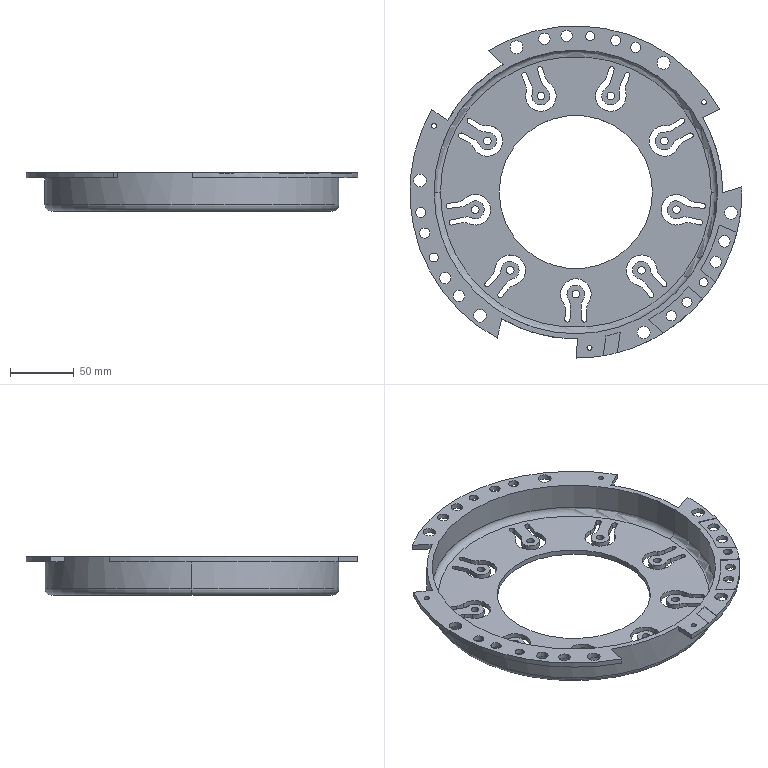Part | SolidWorks | features ICE 7, Fillet 2, Extrusion 1, Shell 1 | 1 solid | 242 faces | box 260 x 260 x 30 mm | volume 210194 mm3 | cylinder 181 | plane 57 | torus 4 | commonest cylinder face diameters 20 x40 4 x32 6 x18 14 x18 24 x18 8 x12